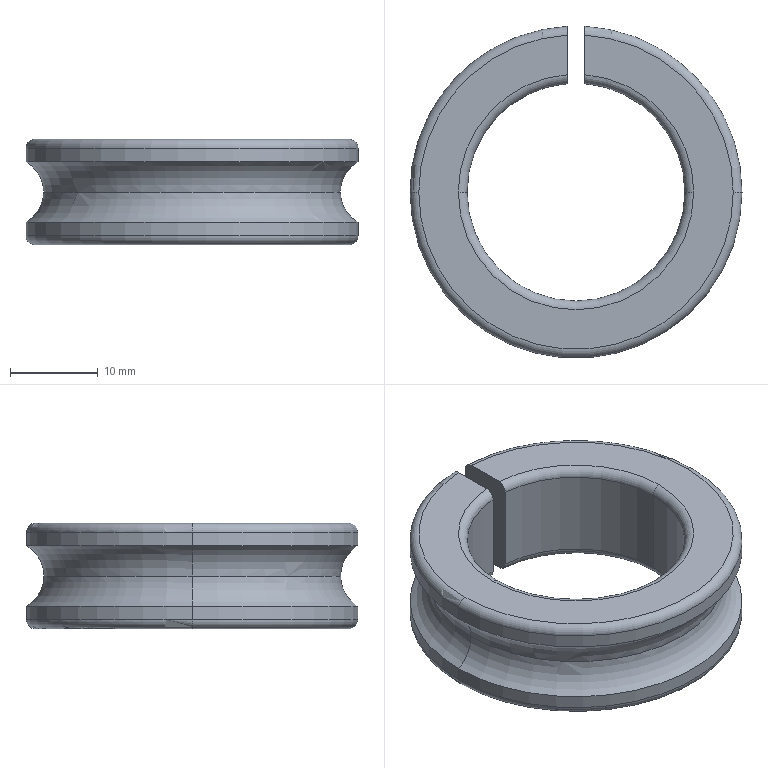Part | STEP file | 10000020543swp000-1 | 1 solid | 31 faces | box 37.8 x 37.774 x 12 mm | volume 6334 mm3 | torus 18 | cylinder 9 | plane 4 | commonest cylinder face diameters 37.8 x6 24.8 x3
STEP:
#1=CARTESIAN_POINT('',(-1.,16.87,0.));
#2=VERTEX_POINT('',#1);
#3=CARTESIAN_POINT('',(-1.,18.874,3.464));
#4=VERTEX_POINT('',#3);
#5=CARTESIAN_POINT('',(-1.,16.87,0.));
#6=CARTESIAN_POINT('',(-1.,16.87,0.3477));
#7=CARTESIAN_POINT('',(-1.,16.917,0.701));
#8=CARTESIAN_POINT('',(-1.,17.053,1.205));
#9=CARTESIAN_POINT('',(-1.,17.109,1.37));
#10=CARTESIAN_POINT('',(-1.,17.242,1.692));
#11=CARTESIAN_POINT('',(-1.,17.321,1.85));
#12=CARTESIAN_POINT('',(-1.,17.584,2.305));
#13=CARTESIAN_POINT('',(-1.,17.796,2.581));
#14=CARTESIAN_POINT('',(-1.,18.168,2.953));
#15=CARTESIAN_POINT('',(-1.,18.301,3.069));
#16=CARTESIAN_POINT('',(-1.,18.578,3.281));
#17=CARTESIAN_POINT('',(-1.,18.723,3.377));
#18=CARTESIAN_POINT('',(-1.,18.874,3.464));
#19=B_SPLINE_CURVE_WITH_KNOTS('',3,(#5,#6,#7,#8,#9,#10,#11,#12,#13,#14,#15,#16,#17,#18),.UNSPECIFIED.,.F.,.F.,(4,2,2,2,2,2,4),(0.002107,0.00315,0.003671,0.004193,0.005236,0.005757,0.006279),.UNSPECIFIED.);
#20=EDGE_CURVE('',#2,#4,#19,.T.);
#21=ORIENTED_EDGE('',*,*,#20,.F.);
#22=CARTESIAN_POINT('',(-16.9,0.,0.));
#23=VERTEX_POINT('',#22);
#24=CARTESIAN_POINT('',(0.,0.,0.));
#25=DIRECTION('',(0.,0.,1.));
#26=DIRECTION('',(1.,0.,0.));
#27=AXIS2_PLACEMENT_3D('',#24,#25,#26);
#28=CIRCLE('',#27,16.9);
#29=EDGE_CURVE('',#2,#23,#28,.T.);
#30=ORIENTED_EDGE('',*,*,#29,.T.);
#31=CARTESIAN_POINT('',(-18.9,0.,3.464));
#32=VERTEX_POINT('',#31);
#33=CARTESIAN_POINT('',(-20.9,0.,0.));
#34=DIRECTION('',(0.,1.,0.));
#35=DIRECTION('',(-1.,0.,0.));
#36=AXIS2_PLACEMENT_3D('',#33,#34,#35);
#37=CIRCLE('',#36,4.);
#38=EDGE_CURVE('',#32,#23,#37,.T.);
#39=ORIENTED_EDGE('',*,*,#38,.F.);
#40=CARTESIAN_POINT('',(0.,0.,3.464));
#41=DIRECTION('',(0.,0.,-1.));
#42=DIRECTION('',(-1.,0.,0.));
#43=AXIS2_PLACEMENT_3D('',#40,#41,#42);
#44=CIRCLE('',#43,18.9);
#45=EDGE_CURVE('',#32,#4,#44,.T.);
#46=ORIENTED_EDGE('',*,*,#45,.T.);
#47=EDGE_LOOP('',(#21,#30,#39,#46));
#48=FACE_OUTER_BOUND('',#47,.T.);
#49=CARTESIAN_POINT('',(0.,0.,0.));
#50=DIRECTION('',(0.,0.,1.));
#51=DIRECTION('',(1.,0.,0.));
#52=AXIS2_PLACEMENT_3D('',#49,#50,#51);
#53=TOROIDAL_SURFACE('',#52,20.9,4.);
#54=ADVANCED_FACE('',(#48),#53,.F.);
#55=CARTESIAN_POINT('',(18.9,0.,3.464));
#56=VERTEX_POINT('',#55);
#57=CARTESIAN_POINT('',(16.9,0.,0.));
#58=VERTEX_POINT('',#57);
#59=CARTESIAN_POINT('',(20.9,0.,0.));
#60=DIRECTION('',(0.,-1.,0.));
#61=DIRECTION('',(0.,0.,-1.));
#62=AXIS2_PLACEMENT_3D('',#59,#60,#61);
#63=CIRCLE('',#62,4.);
#64=EDGE_CURVE('',#56,#58,#63,.T.);
#65=ORIENTED_EDGE('',*,*,#64,.T.);
#66=CARTESIAN_POINT('',(1.,16.87,0.));
#67=VERTEX_POINT('',#66);
#68=CARTESIAN_POINT('',(0.,0.,0.));
#69=DIRECTION('',(0.,0.,1.));
#70=DIRECTION('',(1.,0.,0.));
#71=AXIS2_PLACEMENT_3D('',#68,#69,#70);
#72=CIRCLE('',#71,16.9);
#73=EDGE_CURVE('',#58,#67,#72,.T.);
#74=ORIENTED_EDGE('',*,*,#73,.T.);
#75=CARTESIAN_POINT('',(1.,18.874,3.464));
#76=VERTEX_POINT('',#75);
#77=CARTESIAN_POINT('',(1.,18.874,3.464));
#78=CARTESIAN_POINT('',(1.,18.569,3.289));
#79=CARTESIAN_POINT('',(1.,18.292,3.076));
#80=CARTESIAN_POINT('',(1.,17.922,2.706));
#81=CARTESIAN_POINT('',(1.,17.805,2.574));
#82=CARTESIAN_POINT('',(1.,17.591,2.296));
#83=CARTESIAN_POINT('',(1.,17.398,2.006));
#84=CARTESIAN_POINT('',(1.,17.243,1.694));
#85=CARTESIAN_POINT('',(1.,17.109,1.371));
#86=CARTESIAN_POINT('',(1.,17.052,1.203));
#87=CARTESIAN_POINT('',(1.,16.917,0.6983));
#88=CARTESIAN_POINT('',(1.,16.87,0.3515));
#89=CARTESIAN_POINT('',(1.,16.87,0.));
#90=B_SPLINE_CURVE_WITH_KNOTS('',3,(#77,#78,#79,#80,#81,#82,#83,#84,#85,#86,#87,#88,#89),.UNSPECIFIED.,.F.,.F.,(4,2,2,1,2,2,4),(0.01875,0.01979,0.02031,0.02084,0.02136,0.02188,0.02292),.UNSPECIFIED.);
#91=EDGE_CURVE('',#76,#67,#90,.T.);
#92=ORIENTED_EDGE('',*,*,#91,.F.);
#93=CARTESIAN_POINT('',(0.,0.,3.464));
#94=DIRECTION('',(0.,0.,-1.));
#95=DIRECTION('',(-1.,0.,0.));
#96=AXIS2_PLACEMENT_3D('',#93,#94,#95);
#97=CIRCLE('',#96,18.9);
#98=EDGE_CURVE('',#76,#56,#97,.T.);
#99=ORIENTED_EDGE('',*,*,#98,.T.);
#100=EDGE_LOOP('',(#65,#74,#92,#99));
#101=FACE_OUTER_BOUND('',#100,.T.);
#102=CARTESIAN_POINT('',(0.,0.,0.));
#103=DIRECTION('',(0.,0.,1.));
#104=DIRECTION('',(1.,0.,0.));
#105=AXIS2_PLACEMENT_3D('',#102,#103,#104);
#106=TOROIDAL_SURFACE('',#105,20.9,4.);
#107=ADVANCED_FACE('',(#101),#106,.F.);
#108=ORIENTED_EDGE('',*,*,#38,.T.);
#109=CARTESIAN_POINT('',(0.,0.,0.));
#110=DIRECTION('',(0.,0.,1.));
#111=DIRECTION('',(1.,0.,0.));
#112=AXIS2_PLACEMENT_3D('',#109,#110,#111);
#113=CIRCLE('',#112,16.9);
#114=EDGE_CURVE('',#23,#58,#113,.T.);
#115=ORIENTED_EDGE('',*,*,#114,.T.);
#116=ORIENTED_EDGE('',*,*,#64,.F.);
#117=CARTESIAN_POINT('',(0.,0.,3.464));
#118=DIRECTION('',(0.,0.,-1.));
#119=DIRECTION('',(-1.,0.,0.));
#120=AXIS2_PLACEMENT_3D('',#117,#118,#119);
#121=CIRCLE('',#120,18.9);
#122=EDGE_CURVE('',#56,#32,#121,.T.);
#123=ORIENTED_EDGE('',*,*,#122,.T.);
#124=EDGE_LOOP('',(#108,#115,#116,#123));
#125=FACE_OUTER_BOUND('',#124,.T.);
#126=CARTESIAN_POINT('',(0.,0.,0.));
#127=DIRECTION('',(0.,0.,1.));
#128=DIRECTION('',(1.,0.,0.));
#129=AXIS2_PLACEMENT_3D('',#126,#127,#128);
#130=TOROIDAL_SURFACE('',#129,20.9,4.);
#131=ADVANCED_FACE('',(#125),#130,.F.);
#132=CARTESIAN_POINT('',(-17.9,0.,-6.));
#133=VERTEX_POINT('',#132);
#134=CARTESIAN_POINT('',(-1.,17.872,-6.));
#135=VERTEX_POINT('',#134);
#136=CARTESIAN_POINT('',(0.,0.,-6.));
#137=DIRECTION('',(0.,0.,-1.));
#138=DIRECTION('',(1.,0.,0.));
#139=AXIS2_PLACEMENT_3D('',#136,#137,#138);
#140=CIRCLE('',#139,17.9);
#141=EDGE_CURVE('',#133,#135,#140,.T.);
#142=ORIENTED_EDGE('',*,*,#141,.F.);
#143=CARTESIAN_POINT('',(-18.9,0.,-5.));
#144=VERTEX_POINT('',#143);
#145=CARTESIAN_POINT('',(-17.9,0.,-5.));
#146=DIRECTION('',(0.,1.,0.));
#147=DIRECTION('',(-1.,0.,0.));
#148=AXIS2_PLACEMENT_3D('',#145,#146,#147);
#149=CIRCLE('',#148,1.);
#150=EDGE_CURVE('',#133,#144,#149,.T.);
#151=ORIENTED_EDGE('',*,*,#150,.T.);
#152=CARTESIAN_POINT('',(-1.,18.874,-5.));
#153=VERTEX_POINT('',#152);
#154=CARTESIAN_POINT('',(0.,0.,-5.));
#155=DIRECTION('',(0.,0.,1.));
#156=DIRECTION('',(1.,0.,0.));
#157=AXIS2_PLACEMENT_3D('',#154,#155,#156);
#158=CIRCLE('',#157,18.9);
#159=EDGE_CURVE('',#153,#144,#158,.T.);
#160=ORIENTED_EDGE('',*,*,#159,.F.);
#161=CARTESIAN_POINT('',(-1.,17.872,-6.));
#162=CARTESIAN_POINT('',(-1.,18.004,-6.));
#163=CARTESIAN_POINT('',(-1.,18.134,-5.974));
#164=CARTESIAN_POINT('',(-1.,18.376,-5.874));
#165=CARTESIAN_POINT('',(-1.,18.487,-5.8));
#166=CARTESIAN_POINT('',(-1.,18.765,-5.523));
#167=CARTESIAN_POINT('',(-1.,18.874,-5.264));
#168=CARTESIAN_POINT('',(-1.,18.874,-5.));
#169=B_SPLINE_CURVE_WITH_KNOTS('',3,(#161,#162,#163,#164,#165,#166,#167,#168),.UNSPECIFIED.,.F.,.F.,(4,2,2,4),(0.,0.0003908,0.0007817,0.001563),.UNSPECIFIED.);
#170=EDGE_CURVE('',#135,#153,#169,.T.);
#171=ORIENTED_EDGE('',*,*,#170,.F.);
#172=EDGE_LOOP('',(#142,#151,#160,#171));
#173=FACE_OUTER_BOUND('',#172,.T.);
#174=CARTESIAN_POINT('',(0.,0.,-5.));
#175=DIRECTION('',(0.,0.,1.));
#176=DIRECTION('',(1.,0.,0.));
#177=AXIS2_PLACEMENT_3D('',#174,#175,#176);
#178=TOROIDAL_SURFACE('',#177,17.9,1.);
#179=ADVANCED_FACE('',(#173),#178,.T.);
#180=ORIENTED_EDGE('',*,*,#150,.F.);
#181=CARTESIAN_POINT('',(17.9,0.,-6.));
#182=VERTEX_POINT('',#181);
#183=CARTESIAN_POINT('',(0.,0.,-6.));
#184=DIRECTION('',(0.,0.,-1.));
#185=DIRECTION('',(1.,0.,0.));
#186=AXIS2_PLACEMENT_3D('',#183,#184,#185);
#187=CIRCLE('',#186,17.9);
#188=EDGE_CURVE('',#182,#133,#187,.T.);
#189=ORIENTED_EDGE('',*,*,#188,.F.);
#190=CARTESIAN_POINT('',(18.9,0.,-5.));
#191=VERTEX_POINT('',#190);
#192=CARTESIAN_POINT('',(17.9,0.,-5.));
#193=DIRECTION('',(0.,-1.,0.));
#194=DIRECTION('',(0.,0.,-1.));
#195=AXIS2_PLACEMENT_3D('',#192,#193,#194);
#196=CIRCLE('',#195,1.);
#197=EDGE_CURVE('',#182,#191,#196,.T.);
#198=ORIENTED_EDGE('',*,*,#197,.T.);
#199=CARTESIAN_POINT('',(0.,0.,-5.));
#200=DIRECTION('',(0.,0.,1.));
#201=DIRECTION('',(1.,0.,0.));
#202=AXIS2_PLACEMENT_3D('',#199,#200,#201);
#203=CIRCLE('',#202,18.9);
#204=EDGE_CURVE('',#144,#191,#203,.T.);
#205=ORIENTED_EDGE('',*,*,#204,.F.);
#206=EDGE_LOOP('',(#180,#189,#198,#205));
#207=FACE_OUTER_BOUND('',#206,.T.);
#208=CARTESIAN_POINT('',(0.,0.,-5.));
#209=DIRECTION('',(0.,0.,1.));
#210=DIRECTION('',(1.,0.,0.));
#211=AXIS2_PLACEMENT_3D('',#208,#209,#210);
#212=TOROIDAL_SURFACE('',#211,17.9,1.);
#213=ADVANCED_FACE('',(#207),#212,.T.);
#214=CARTESIAN_POINT('',(-12.4,0.,-5.));
#215=VERTEX_POINT('',#214);
#216=CARTESIAN_POINT('',(-1.,12.36,-5.));
#217=VERTEX_POINT('',#216);
#218=CARTESIAN_POINT('',(0.,0.,-5.));
#219=DIRECTION('',(0.,0.,-1.));
#220=DIRECTION('',(1.,0.,0.));
#221=AXIS2_PLACEMENT_3D('',#218,#219,#220);
#222=CIRCLE('',#221,12.4);
#223=EDGE_CURVE('',#215,#217,#222,.T.);
#224=ORIENTED_EDGE('',*,*,#223,.F.);
#225=CARTESIAN_POINT('',(-13.4,0.,-6.));
#226=VERTEX_POINT('',#225);
#227=CARTESIAN_POINT('',(-13.4,0.,-5.));
#228=DIRECTION('',(0.,1.,0.));
#229=DIRECTION('',(-1.,0.,0.));
#230=AXIS2_PLACEMENT_3D('',#227,#228,#229);
#231=CIRCLE('',#230,1.);
#232=EDGE_CURVE('',#215,#226,#231,.T.);
#233=ORIENTED_EDGE('',*,*,#232,.T.);
#234=CARTESIAN_POINT('',(-1.,13.363,-6.));
#235=VERTEX_POINT('',#234);
#236=CARTESIAN_POINT('',(0.,0.,-6.));
#237=DIRECTION('',(0.,0.,1.));
#238=DIRECTION('',(1.,0.,0.));
#239=AXIS2_PLACEMENT_3D('',#236,#237,#238);
#240=CIRCLE('',#239,13.4);
#241=EDGE_CURVE('',#235,#226,#240,.T.);
#242=ORIENTED_EDGE('',*,*,#241,.F.);
#243=CARTESIAN_POINT('',(-1.,12.36,-5.));
#244=CARTESIAN_POINT('',(-1.,12.36,-5.132));
#245=CARTESIAN_POINT('',(-1.,12.386,-5.262));
#246=CARTESIAN_POINT('',(-1.,12.487,-5.504));
#247=CARTESIAN_POINT('',(-1.,12.561,-5.615));
#248=CARTESIAN_POINT('',(-1.,12.839,-5.892));
#249=CARTESIAN_POINT('',(-1.,13.098,-6.));
#250=CARTESIAN_POINT('',(-1.,13.363,-6.));
#251=B_SPLINE_CURVE_WITH_KNOTS('',3,(#243,#244,#245,#246,#247,#248,#249,#250),.UNSPECIFIED.,.F.,.F.,(4,2,2,4),(0.,0.0003911,0.0007822,0.001564),.UNSPECIFIED.);
#252=EDGE_CURVE('',#217,#235,#251,.T.);
#253=ORIENTED_EDGE('',*,*,#252,.F.);
#254=EDGE_LOOP('',(#224,#233,#242,#253));
#255=FACE_OUTER_BOUND('',#254,.T.);
#256=CARTESIAN_POINT('',(0.,0.,-5.));
#257=DIRECTION('',(0.,0.,1.));
#258=DIRECTION('',(1.,0.,0.));
#259=AXIS2_PLACEMENT_3D('',#256,#257,#258);
#260=TOROIDAL_SURFACE('',#259,13.4,1.);
#261=ADVANCED_FACE('',(#255),#260,.T.);
#262=ORIENTED_EDGE('',*,*,#232,.F.);
#263=CARTESIAN_POINT('',(12.4,0.,-5.));
#264=VERTEX_POINT('',#263);
#265=CARTESIAN_POINT('',(0.,0.,-5.));
#266=DIRECTION('',(0.,0.,-1.));
#267=DIRECTION('',(1.,0.,0.));
#268=AXIS2_PLACEMENT_3D('',#265,#266,#267);
#269=CIRCLE('',#268,12.4);
#270=EDGE_CURVE('',#264,#215,#269,.T.);
#271=ORIENTED_EDGE('',*,*,#270,.F.);
#272=CARTESIAN_POINT('',(13.4,0.,-6.));
#273=VERTEX_POINT('',#272);
#274=CARTESIAN_POINT('',(13.4,0.,-5.));
#275=DIRECTION('',(0.,-1.,0.));
#276=DIRECTION('',(0.,0.,-1.));
#277=AXIS2_PLACEMENT_3D('',#274,#275,#276);
#278=CIRCLE('',#277,1.);
#279=EDGE_CURVE('',#264,#273,#278,.T.);
#280=ORIENTED_EDGE('',*,*,#279,.T.);
#281=CARTESIAN_POINT('',(0.,0.,-6.));
#282=DIRECTION('',(0.,0.,1.));
#283=DIRECTION('',(1.,0.,0.));
#284=AXIS2_PLACEMENT_3D('',#281,#282,#283);
#285=CIRCLE('',#284,13.4);
#286=EDGE_CURVE('',#226,#273,#285,.T.);
#287=ORIENTED_EDGE('',*,*,#286,.F.);
#288=EDGE_LOOP('',(#262,#271,#280,#287));
#289=FACE_OUTER_BOUND('',#288,.T.);
#290=CARTESIAN_POINT('',(0.,0.,-5.));
#291=DIRECTION('',(0.,0.,1.));
#292=DIRECTION('',(1.,0.,0.));
#293=AXIS2_PLACEMENT_3D('',#290,#291,#292);
#294=TOROIDAL_SURFACE('',#293,13.4,1.);
#295=ADVANCED_FACE('',(#289),#294,.T.);
#296=CARTESIAN_POINT('',(-13.4,0.,6.));
#297=VERTEX_POINT('',#296);
#298=CARTESIAN_POINT('',(-1.,13.363,6.));
#299=VERTEX_POINT('',#298);
#300=CARTESIAN_POINT('',(0.,0.,6.));
#301=DIRECTION('',(0.,0.,-1.));
#302=DIRECTION('',(1.,0.,0.));
#303=AXIS2_PLACEMENT_3D('',#300,#301,#302);
#304=CIRCLE('',#303,13.4);
#305=EDGE_CURVE('',#297,#299,#304,.T.);
#306=ORIENTED_EDGE('',*,*,#305,.F.);
#307=CARTESIAN_POINT('',(-12.4,0.,5.));
#308=VERTEX_POINT('',#307);
#309=CARTESIAN_POINT('',(-13.4,0.,5.));
#310=DIRECTION('',(0.,1.,0.));
#311=DIRECTION('',(-1.,0.,0.));
#312=AXIS2_PLACEMENT_3D('',#309,#310,#311);
#313=CIRCLE('',#312,1.);
#314=EDGE_CURVE('',#297,#308,#313,.T.);
#315=ORIENTED_EDGE('',*,*,#314,.T.);
#316=CARTESIAN_POINT('',(-1.,12.36,5.));
#317=VERTEX_POINT('',#316);
#318=CARTESIAN_POINT('',(0.,0.,5.));
#319=DIRECTION('',(0.,0.,1.));
#320=DIRECTION('',(1.,0.,0.));
#321=AXIS2_PLACEMENT_3D('',#318,#319,#320);
#322=CIRCLE('',#321,12.4);
#323=EDGE_CURVE('',#317,#308,#322,.T.);
#324=ORIENTED_EDGE('',*,*,#323,.F.);
#325=CARTESIAN_POINT('',(-1.,13.363,6.));
#326=CARTESIAN_POINT('',(-1.,13.23,6.));
#327=CARTESIAN_POINT('',(-1.,13.101,5.974));
#328=CARTESIAN_POINT('',(-1.,12.858,5.874));
#329=CARTESIAN_POINT('',(-1.,12.747,5.8));
#330=CARTESIAN_POINT('',(-1.,12.469,5.524));
#331=CARTESIAN_POINT('',(-1.,12.36,5.265));
#332=CARTESIAN_POINT('',(-1.,12.36,5.));
#333=B_SPLINE_CURVE_WITH_KNOTS('',3,(#325,#326,#327,#328,#329,#330,#331,#332),.UNSPECIFIED.,.F.,.F.,(4,2,2,4),(0.,0.0003911,0.0007822,0.001564),.UNSPECIFIED.);
#334=EDGE_CURVE('',#299,#317,#333,.T.);
#335=ORIENTED_EDGE('',*,*,#334,.F.);
#336=EDGE_LOOP('',(#306,#315,#324,#335));
#337=FACE_OUTER_BOUND('',#336,.T.);
#338=CARTESIAN_POINT('',(0.,0.,5.));
#339=DIRECTION('',(0.,0.,1.));
#340=DIRECTION('',(1.,0.,0.));
#341=AXIS2_PLACEMENT_3D('',#338,#339,#340);
#342=TOROIDAL_SURFACE('',#341,13.4,1.);
#343=ADVANCED_FACE('',(#337),#342,.T.);
#344=ORIENTED_EDGE('',*,*,#314,.F.);
#345=CARTESIAN_POINT('',(13.4,0.,6.));
#346=VERTEX_POINT('',#345);
#347=CARTESIAN_POINT('',(0.,0.,6.));
#348=DIRECTION('',(0.,0.,-1.));
#349=DIRECTION('',(1.,0.,0.));
#350=AXIS2_PLACEMENT_3D('',#347,#348,#349);
#351=CIRCLE('',#350,13.4);
#352=EDGE_CURVE('',#346,#297,#351,.T.);
#353=ORIENTED_EDGE('',*,*,#352,.F.);
#354=CARTESIAN_POINT('',(12.4,0.,5.));
#355=VERTEX_POINT('',#354);
#356=CARTESIAN_POINT('',(13.4,0.,5.));
#357=DIRECTION('',(0.,-1.,0.));
#358=DIRECTION('',(0.,0.,-1.));
#359=AXIS2_PLACEMENT_3D('',#356,#357,#358);
#360=CIRCLE('',#359,1.);
#361=EDGE_CURVE('',#346,#355,#360,.T.);
#362=ORIENTED_EDGE('',*,*,#361,.T.);
#363=CARTESIAN_POINT('',(0.,0.,5.));
#364=DIRECTION('',(0.,0.,1.));
#365=DIRECTION('',(1.,0.,0.));
#366=AXIS2_PLACEMENT_3D('',#363,#364,#365);
#367=CIRCLE('',#366,12.4);
#368=EDGE_CURVE('',#308,#355,#367,.T.);
#369=ORIENTED_EDGE('',*,*,#368,.F.);
#370=EDGE_LOOP('',(#344,#353,#362,#369));
#371=FACE_OUTER_BOUND('',#370,.T.);
#372=CARTESIAN_POINT('',(0.,0.,5.));
#373=DIRECTION('',(0.,0.,1.));
#374=DIRECTION('',(1.,0.,0.));
#375=AXIS2_PLACEMENT_3D('',#372,#373,#374);
#376=TOROIDAL_SURFACE('',#375,13.4,1.);
#377=ADVANCED_FACE('',(#371),#376,.T.);
#378=CARTESIAN_POINT('',(-18.9,0.,5.));
#379=VERTEX_POINT('',#378);
#380=CARTESIAN_POINT('',(-1.,18.874,5.));
#381=VERTEX_POINT('',#380);
#382=CARTESIAN_POINT('',(0.,0.,5.));
#383=DIRECTION('',(0.,0.,-1.));
#384=DIRECTION('',(1.,0.,0.));
#385=AXIS2_PLACEMENT_3D('',#382,#383,#384);
#386=CIRCLE('',#385,18.9);
#387=EDGE_CURVE('',#379,#381,#386,.T.);
#388=ORIENTED_EDGE('',*,*,#387,.F.);
#389=CARTESIAN_POINT('',(-17.9,0.,6.));
#390=VERTEX_POINT('',#389);
#391=CARTESIAN_POINT('',(-17.9,0.,5.));
#392=DIRECTION('',(0.,1.,0.));
#393=DIRECTION('',(-1.,0.,0.));
#394=AXIS2_PLACEMENT_3D('',#391,#392,#393);
#395=CIRCLE('',#394,1.);
#396=EDGE_CURVE('',#379,#390,#395,.T.);
#397=ORIENTED_EDGE('',*,*,#396,.T.);
#398=CARTESIAN_POINT('',(-1.,17.872,6.));
#399=VERTEX_POINT('',#398);
#400=CARTESIAN_POINT('',(0.,0.,6.));
#401=DIRECTION('',(0.,0.,1.));
#402=DIRECTION('',(1.,0.,0.));
#403=AXIS2_PLACEMENT_3D('',#400,#401,#402);
#404=CIRCLE('',#403,17.9);
#405=EDGE_CURVE('',#399,#390,#404,.T.);
#406=ORIENTED_EDGE('',*,*,#405,.F.);
#407=CARTESIAN_POINT('',(-1.,18.874,5.));
#408=CARTESIAN_POINT('',(-1.,18.874,5.132));
#409=CARTESIAN_POINT('',(-1.,18.847,5.262));
#410=CARTESIAN_POINT('',(-1.,18.747,5.504));
#411=CARTESIAN_POINT('',(-1.,18.673,5.615));
#412=CARTESIAN_POINT('',(-1.,18.396,5.892));
#413=CARTESIAN_POINT('',(-1.,18.136,6.));
#414=CARTESIAN_POINT('',(-1.,17.872,6.));
#415=B_SPLINE_CURVE_WITH_KNOTS('',3,(#407,#408,#409,#410,#411,#412,#413,#414),.UNSPECIFIED.,.F.,.F.,(4,2,2,4),(0.,0.0003908,0.0007817,0.001563),.UNSPECIFIED.);
#416=EDGE_CURVE('',#381,#399,#415,.T.);
#417=ORIENTED_EDGE('',*,*,#416,.F.);
#418=EDGE_LOOP('',(#388,#397,#406,#417));
#419=FACE_OUTER_BOUND('',#418,.T.);
#420=CARTESIAN_POINT('',(0.,0.,5.));
#421=DIRECTION('',(0.,0.,1.));
#422=DIRECTION('',(1.,0.,0.));
#423=AXIS2_PLACEMENT_3D('',#420,#421,#422);
#424=TOROIDAL_SURFACE('',#423,17.9,1.);
#425=ADVANCED_FACE('',(#419),#424,.T.);
#426=ORIENTED_EDGE('',*,*,#396,.F.);
#427=CARTESIAN_POINT('',(18.9,0.,5.));
#428=VERTEX_POINT('',#427);
#429=CARTESIAN_POINT('',(0.,0.,5.));
#430=DIRECTION('',(0.,0.,-1.));
#431=DIRECTION('',(1.,0.,0.));
#432=AXIS2_PLACEMENT_3D('',#429,#430,#431);
#433=CIRCLE('',#432,18.9);
#434=EDGE_CURVE('',#428,#379,#433,.T.);
#435=ORIENTED_EDGE('',*,*,#434,.F.);
#436=CARTESIAN_POINT('',(17.9,0.,6.));
#437=VERTEX_POINT('',#436);
#438=CARTESIAN_POINT('',(17.9,0.,5.));
#439=DIRECTION('',(0.,-1.,0.));
#440=DIRECTION('',(0.,0.,-1.));
#441=AXIS2_PLACEMENT_3D('',#438,#439,#440);
#442=CIRCLE('',#441,1.);
#443=EDGE_CURVE('',#428,#437,#442,.T.);
#444=ORIENTED_EDGE('',*,*,#443,.T.);
#445=CARTESIAN_POINT('',(0.,0.,6.));
#446=DIRECTION('',(0.,0.,1.));
#447=DIRECTION('',(1.,0.,0.));
#448=AXIS2_PLACEMENT_3D('',#445,#446,#447);
#449=CIRCLE('',#448,17.9);
#450=EDGE_CURVE('',#390,#437,#449,.T.);
#451=ORIENTED_EDGE('',*,*,#450,.F.);
#452=EDGE_LOOP('',(#426,#435,#444,#451));
#453=FACE_OUTER_BOUND('',#452,.T.);
#454=CARTESIAN_POINT('',(0.,0.,5.));
#455=DIRECTION('',(0.,0.,1.));
#456=DIRECTION('',(1.,0.,0.));
#457=AXIS2_PLACEMENT_3D('',#454,#455,#456);
#458=TOROIDAL_SURFACE('',#457,17.9,1.);
#459=ADVANCED_FACE('',(#453),#458,.T.);
#460=ORIENTED_EDGE('',*,*,#114,.F.);
#461=CARTESIAN_POINT('',(-18.9,0.,-3.464));
#462=VERTEX_POINT('',#461);
#463=CARTESIAN_POINT('',(-20.9,0.,0.));
#464=DIRECTION('',(0.,1.,0.));
#465=DIRECTION('',(-1.,0.,0.));
#466=AXIS2_PLACEMENT_3D('',#463,#464,#465);
#467=CIRCLE('',#466,4.);
#468=EDGE_CURVE('',#23,#462,#467,.T.);
#469=ORIENTED_EDGE('',*,*,#468,.T.);
#470=CARTESIAN_POINT('',(18.9,0.,-3.464));
#471=VERTEX_POINT('',#470);
#472=CARTESIAN_POINT('',(0.,0.,-3.464));
#473=DIRECTION('',(0.,0.,1.));
#474=DIRECTION('',(1.,0.,0.));
#475=AXIS2_PLACEMENT_3D('',#472,#473,#474);
#476=CIRCLE('',#475,18.9);
#477=EDGE_CURVE('',#462,#471,#476,.T.);
#478=ORIENTED_EDGE('',*,*,#477,.T.);
#479=CARTESIAN_POINT('',(20.9,0.,0.));
#480=DIRECTION('',(0.,-1.,0.));
#481=DIRECTION('',(0.,0.,-1.));
#482=AXIS2_PLACEMENT_3D('',#479,#480,#481);
#483=CIRCLE('',#482,4.);
#484=EDGE_CURVE('',#58,#471,#483,.T.);
#485=ORIENTED_EDGE('',*,*,#484,.F.);
#486=EDGE_LOOP('',(#460,#469,#478,#485));
#487=FACE_OUTER_BOUND('',#486,.T.);
#488=CARTESIAN_POINT('',(0.,0.,0.));
#489=DIRECTION('',(0.,0.,1.));
#490=DIRECTION('',(1.,0.,0.));
#491=AXIS2_PLACEMENT_3D('',#488,#489,#490);
#492=TOROIDAL_SURFACE('',#491,20.9,4.);
#493=ADVANCED_FACE('',(#487),#492,.F.);
#494=ORIENTED_EDGE('',*,*,#73,.F.);
#495=ORIENTED_EDGE('',*,*,#484,.T.);
#496=CARTESIAN_POINT('',(1.,18.874,-3.464));
#497=VERTEX_POINT('',#496);
#498=CARTESIAN_POINT('',(0.,0.,-3.464));
#499=DIRECTION('',(0.,0.,1.));
#500=DIRECTION('',(1.,0.,0.));
#501=AXIS2_PLACEMENT_3D('',#498,#499,#500);
#502=CIRCLE('',#501,18.9);
#503=EDGE_CURVE('',#471,#497,#502,.T.);
#504=ORIENTED_EDGE('',*,*,#503,.T.);
#505=CARTESIAN_POINT('',(1.,16.87,0.));
#506=CARTESIAN_POINT('',(1.,16.87,-0.3513));
#507=CARTESIAN_POINT('',(1.,16.916,-0.6956));
#508=CARTESIAN_POINT('',(1.,17.051,-1.202));
#509=CARTESIAN_POINT('',(1.,17.108,-1.369));
#510=CARTESIAN_POINT('',(1.,17.243,-1.693));
#511=CARTESIAN_POINT('',(1.,17.32,-1.85));
#512=CARTESIAN_POINT('',(1.,17.585,-2.307));
#513=CARTESIAN_POINT('',(1.,17.798,-2.583));
#514=CARTESIAN_POINT('',(1.,18.168,-2.952));
#515=CARTESIAN_POINT('',(1.,18.301,-3.068));
#516=CARTESIAN_POINT('',(1.,18.578,-3.281));
#517=CARTESIAN_POINT('',(1.,18.723,-3.377));
#518=CARTESIAN_POINT('',(1.,18.874,-3.464));
#519=B_SPLINE_CURVE_WITH_KNOTS('',3,(#505,#506,#507,#508,#509,#510,#511,#512,#513,#514,#515,#516,#517,#518),.UNSPECIFIED.,.F.,.F.,(4,2,2,2,2,2,4),(0.02292,0.02396,0.02448,0.025,0.02605,0.02657,0.02709),.UNSPECIFIED.);
#520=EDGE_CURVE('',#67,#497,#519,.T.);
#521=ORIENTED_EDGE('',*,*,#520,.F.);
#522=EDGE_LOOP('',(#494,#495,#504,#521));
#523=FACE_OUTER_BOUND('',#522,.T.);
#524=CARTESIAN_POINT('',(0.,0.,0.));
#525=DIRECTION('',(0.,0.,1.));
#526=DIRECTION('',(1.,0.,0.));
#527=AXIS2_PLACEMENT_3D('',#524,#525,#526);
#528=TOROIDAL_SURFACE('',#527,20.9,4.);
#529=ADVANCED_FACE('',(#523),#528,.F.);
#530=ORIENTED_EDGE('',*,*,#368,.T.);
#531=CARTESIAN_POINT('',(12.4,0.,6.));
#532=DIRECTION('',(0.,0.,-1.));
#533=VECTOR('',#532,1000.);
#534=LINE('',#531,#533);
#535=EDGE_CURVE('',#355,#264,#534,.T.);
#536=ORIENTED_EDGE('',*,*,#535,.T.);
#537=ORIENTED_EDGE('',*,*,#270,.T.);
#538=CARTESIAN_POINT('',(-12.4,0.,6.));
#539=DIRECTION('',(0.,0.,-1.));
#540=VECTOR('',#539,1000.);
#541=LINE('',#538,#540);
#542=EDGE_CURVE('',#308,#215,#541,.T.);
#543=ORIENTED_EDGE('',*,*,#542,.F.);
#544=EDGE_LOOP('',(#530,#536,#537,#543));
#545=FACE_OUTER_BOUND('',#544,.T.);
#546=CARTESIAN_POINT('',(0.,0.,6.));
#547=DIRECTION('',(0.,0.,-1.));
#548=DIRECTION('',(-1.,0.,0.));
#549=AXIS2_PLACEMENT_3D('',#546,#547,#548);
#550=CYLINDRICAL_SURFACE('',#549,12.4);
#551=ADVANCED_FACE('',(#545),#550,.F.);
#552=ORIENTED_EDGE('',*,*,#323,.T.);
#553=ORIENTED_EDGE('',*,*,#542,.T.);
#554=ORIENTED_EDGE('',*,*,#223,.T.);
#555=CARTESIAN_POINT('',(-1.,12.36,6.));
#556=DIRECTION('',(0.,0.,-1.));
#557=VECTOR('',#556,1000.);
#558=LINE('',#555,#557);
#559=EDGE_CURVE('',#317,#217,#558,.T.);
#560=ORIENTED_EDGE('',*,*,#559,.F.);
#561=EDGE_LOOP('',(#552,#553,#554,#560));
#562=FACE_OUTER_BOUND('',#561,.T.);
#563=CARTESIAN_POINT('',(0.,0.,6.));
#564=DIRECTION('',(0.,0.,-1.));
#565=DIRECTION('',(-1.,0.,0.));
#566=AXIS2_PLACEMENT_3D('',#563,#564,#565);
#567=CYLINDRICAL_SURFACE('',#566,12.4);
#568=ADVANCED_FACE('',(#562),#567,.F.);
#569=ORIENTED_EDGE('',*,*,#503,.F.);
#570=CARTESIAN_POINT('',(18.9,0.,6.));
#571=DIRECTION('',(0.,0.,-1.));
#572=VECTOR('',#571,1000.);
#573=LINE('',#570,#572);
#574=EDGE_CURVE('',#471,#191,#573,.T.);
#575=ORIENTED_EDGE('',*,*,#574,.T.);
#576=CARTESIAN_POINT('',(1.,18.874,-5.));
#577=VERTEX_POINT('',#576);
#578=CARTESIAN_POINT('',(0.,0.,-5.));
#579=DIRECTION('',(0.,0.,1.));
#580=DIRECTION('',(1.,0.,0.));
#581=AXIS2_PLACEMENT_3D('',#578,#579,#580);
#582=CIRCLE('',#581,18.9);
#583=EDGE_CURVE('',#191,#577,#582,.T.);
#584=ORIENTED_EDGE('',*,*,#583,.T.);
#585=CARTESIAN_POINT('',(1.,18.874,6.));
#586=DIRECTION('',(0.,0.,-1.));
#587=VECTOR('',#586,1000.);
#588=LINE('',#585,#587);
#589=EDGE_CURVE('',#497,#577,#588,.T.);
#590=ORIENTED_EDGE('',*,*,#589,.F.);
#591=EDGE_LOOP('',(#569,#575,#584,#590));
#592=FACE_OUTER_BOUND('',#591,.T.);
#593=CARTESIAN_POINT('',(0.,0.,6.));
#594=DIRECTION('',(0.,0.,-1.));
#595=DIRECTION('',(-1.,0.,0.));
#596=AXIS2_PLACEMENT_3D('',#593,#594,#595);
#597=CYLINDRICAL_SURFACE('',#596,18.9);
#598=ADVANCED_FACE('',(#592),#597,.T.);
#599=ORIENTED_EDGE('',*,*,#574,.F.);
#600=ORIENTED_EDGE('',*,*,#477,.F.);
#601=CARTESIAN_POINT('',(-18.9,0.,6.));
#602=DIRECTION('',(0.,0.,-1.));
#603=VECTOR('',#602,1000.);
#604=LINE('',#601,#603);
#605=EDGE_CURVE('',#462,#144,#604,.T.);
#606=ORIENTED_EDGE('',*,*,#605,.T.);
#607=ORIENTED_EDGE('',*,*,#204,.T.);
#608=EDGE_LOOP('',(#599,#600,#606,#607));
#609=FACE_OUTER_BOUND('',#608,.T.);
#610=CARTESIAN_POINT('',(0.,0.,6.));
#611=DIRECTION('',(0.,0.,-1.));
#612=DIRECTION('',(-1.,0.,0.));
#613=AXIS2_PLACEMENT_3D('',#610,#611,#612);
#614=CYLINDRICAL_SURFACE('',#613,18.9);
#615=ADVANCED_FACE('',(#609),#614,.T.);
#616=CARTESIAN_POINT('',(1.,18.874,5.));
#617=VERTEX_POINT('',#616);
#618=CARTESIAN_POINT('',(0.,0.,5.));
#619=DIRECTION('',(0.,0.,-1.));
#620=DIRECTION('',(1.,0.,0.));
#621=AXIS2_PLACEMENT_3D('',#618,#619,#620);
#622=CIRCLE('',#621,18.9);
#623=EDGE_CURVE('',#617,#428,#622,.T.);
#624=ORIENTED_EDGE('',*,*,#623,.T.);
#625=CARTESIAN_POINT('',(18.9,0.,6.));
#626=DIRECTION('',(0.,0.,-1.));
#627=VECTOR('',#626,1000.);
#628=LINE('',#625,#627);
#629=EDGE_CURVE('',#428,#56,#628,.T.);
#630=ORIENTED_EDGE('',*,*,#629,.T.);
#631=ORIENTED_EDGE('',*,*,#98,.F.);
#632=CARTESIAN_POINT('',(1.,18.874,6.));
#633=DIRECTION('',(0.,0.,-1.));
#634=VECTOR('',#633,1000.);
#635=LINE('',#632,#634);
#636=EDGE_CURVE('',#617,#76,#635,.T.);
#637=ORIENTED_EDGE('',*,*,#636,.F.);
#638=EDGE_LOOP('',(#624,#630,#631,#637));
#639=FACE_OUTER_BOUND('',#638,.T.);
#640=CARTESIAN_POINT('',(0.,0.,6.));
#641=DIRECTION('',(0.,0.,-1.));
#642=DIRECTION('',(-1.,0.,0.));
#643=AXIS2_PLACEMENT_3D('',#640,#641,#642);
#644=CYLINDRICAL_SURFACE('',#643,18.9);
#645=ADVANCED_FACE('',(#639),#644,.T.);
#646=ORIENTED_EDGE('',*,*,#629,.F.);
#647=ORIENTED_EDGE('',*,*,#434,.T.);
#648=CARTESIAN_POINT('',(-18.9,0.,6.));
#649=DIRECTION('',(0.,0.,-1.));
#650=VECTOR('',#649,1000.);
#651=LINE('',#648,#650);
#652=EDGE_CURVE('',#379,#32,#651,.T.);
#653=ORIENTED_EDGE('',*,*,#652,.T.);
#654=ORIENTED_EDGE('',*,*,#122,.F.);
#655=EDGE_LOOP('',(#646,#647,#653,#654));
#656=FACE_OUTER_BOUND('',#655,.T.);
#657=CARTESIAN_POINT('',(0.,0.,6.));
#658=DIRECTION('',(0.,0.,-1.));
#659=DIRECTION('',(-1.,0.,0.));
#660=AXIS2_PLACEMENT_3D('',#657,#658,#659);
#661=CYLINDRICAL_SURFACE('',#660,18.9);
#662=ADVANCED_FACE('',(#656),#661,.T.);
#663=ORIENTED_EDGE('',*,*,#652,.F.);
#664=ORIENTED_EDGE('',*,*,#387,.T.);
#665=CARTESIAN_POINT('',(-1.,18.874,6.));
#666=DIRECTION('',(0.,0.,-1.));
#667=VECTOR('',#666,1000.);
#668=LINE('',#665,#667);
#669=EDGE_CURVE('',#381,#4,#668,.T.);
#670=ORIENTED_EDGE('',*,*,#669,.T.);
#671=ORIENTED_EDGE('',*,*,#45,.F.);
#672=EDGE_LOOP('',(#663,#664,#670,#671));
#673=FACE_OUTER_BOUND('',#672,.T.);
#674=CARTESIAN_POINT('',(0.,0.,6.));
#675=DIRECTION('',(0.,0.,-1.));
#676=DIRECTION('',(-1.,0.,0.));
#677=AXIS2_PLACEMENT_3D('',#674,#675,#676);
#678=CYLINDRICAL_SURFACE('',#677,18.9);
#679=ADVANCED_FACE('',(#673),#678,.T.);
#680=ORIENTED_EDGE('',*,*,#605,.F.);
#681=CARTESIAN_POINT('',(-1.,18.874,-3.464));
#682=VERTEX_POINT('',#681);
#683=CARTESIAN_POINT('',(0.,0.,-3.464));
#684=DIRECTION('',(0.,0.,1.));
#685=DIRECTION('',(1.,0.,0.));
#686=AXIS2_PLACEMENT_3D('',#683,#684,#685);
#687=CIRCLE('',#686,18.9);
#688=EDGE_CURVE('',#682,#462,#687,.T.);
#689=ORIENTED_EDGE('',*,*,#688,.F.);
#690=CARTESIAN_POINT('',(-1.,18.874,6.));
#691=DIRECTION('',(0.,0.,-1.));
#692=VECTOR('',#691,1000.);
#693=LINE('',#690,#692);
#694=EDGE_CURVE('',#682,#153,#693,.T.);
#695=ORIENTED_EDGE('',*,*,#694,.T.);
#696=ORIENTED_EDGE('',*,*,#159,.T.);
#697=EDGE_LOOP('',(#680,#689,#695,#696));
#698=FACE_OUTER_BOUND('',#697,.T.);
#699=CARTESIAN_POINT('',(0.,0.,6.));
#700=DIRECTION('',(0.,0.,-1.));
#701=DIRECTION('',(-1.,0.,0.));
#702=AXIS2_PLACEMENT_3D('',#699,#700,#701);
#703=CYLINDRICAL_SURFACE('',#702,18.9);
#704=ADVANCED_FACE('',(#698),#703,.T.);
#705=CARTESIAN_POINT('',(-1.,18.874,6.));
#706=DIRECTION('',(0.,1.,0.));
#707=VECTOR('',#706,1000.);
#708=LINE('',#705,#707);
#709=EDGE_CURVE('',#299,#399,#708,.T.);
#710=ORIENTED_EDGE('',*,*,#709,.T.);
#711=ORIENTED_EDGE('',*,*,#405,.T.);
#712=ORIENTED_EDGE('',*,*,#450,.T.);
#713=CARTESIAN_POINT('',(1.,17.872,6.));
#714=VERTEX_POINT('',#713);
#715=CARTESIAN_POINT('',(0.,0.,6.));
#716=DIRECTION('',(0.,0.,1.));
#717=DIRECTION('',(1.,0.,0.));
#718=AXIS2_PLACEMENT_3D('',#715,#716,#717);
#719=CIRCLE('',#718,17.9);
#720=EDGE_CURVE('',#437,#714,#719,.T.);
#721=ORIENTED_EDGE('',*,*,#720,.T.);
#722=CARTESIAN_POINT('',(1.,13.363,6.));
#723=VERTEX_POINT('',#722);
#724=CARTESIAN_POINT('',(1.,18.874,6.));
#725=DIRECTION('',(0.,-1.,0.));
#726=VECTOR('',#725,1000.);
#727=LINE('',#724,#726);
#728=EDGE_CURVE('',#714,#723,#727,.T.);
#729=ORIENTED_EDGE('',*,*,#728,.T.);
#730=CARTESIAN_POINT('',(0.,0.,6.));
#731=DIRECTION('',(0.,0.,-1.));
#732=DIRECTION('',(1.,0.,0.));
#733=AXIS2_PLACEMENT_3D('',#730,#731,#732);
#734=CIRCLE('',#733,13.4);
#735=EDGE_CURVE('',#723,#346,#734,.T.);
#736=ORIENTED_EDGE('',*,*,#735,.T.);
#737=ORIENTED_EDGE('',*,*,#352,.T.);
#738=ORIENTED_EDGE('',*,*,#305,.T.);
#739=EDGE_LOOP('',(#710,#711,#712,#721,#729,#736,#737,#738));
#740=FACE_OUTER_BOUND('',#739,.T.);
#741=CARTESIAN_POINT('',(0.,0.,6.));
#742=DIRECTION('',(0.,0.,1.));
#743=DIRECTION('',(1.,0.,0.));
#744=AXIS2_PLACEMENT_3D('',#741,#742,#743);
#745=PLANE('',#744);
#746=ADVANCED_FACE('',(#740),#745,.T.);
#747=CARTESIAN_POINT('',(-1.,18.874,-6.));
#748=DIRECTION('',(0.,1.,0.));
#749=VECTOR('',#748,1000.);
#750=LINE('',#747,#749);
#751=EDGE_CURVE('',#235,#135,#750,.T.);
#752=ORIENTED_EDGE('',*,*,#751,.F.);
#753=ORIENTED_EDGE('',*,*,#241,.T.);
#754=ORIENTED_EDGE('',*,*,#286,.T.);
#755=CARTESIAN_POINT('',(1.,13.363,-6.));
#756=VERTEX_POINT('',#755);
#757=CARTESIAN_POINT('',(0.,0.,-6.));
#758=DIRECTION('',(0.,0.,1.));
#759=DIRECTION('',(1.,0.,0.));
#760=AXIS2_PLACEMENT_3D('',#757,#758,#759);
#761=CIRCLE('',#760,13.4);
#762=EDGE_CURVE('',#273,#756,#761,.T.);
#763=ORIENTED_EDGE('',*,*,#762,.T.);
#764=CARTESIAN_POINT('',(1.,17.872,-6.));
#765=VERTEX_POINT('',#764);
#766=CARTESIAN_POINT('',(1.,18.874,-6.));
#767=DIRECTION('',(0.,-1.,0.));
#768=VECTOR('',#767,1000.);
#769=LINE('',#766,#768);
#770=EDGE_CURVE('',#765,#756,#769,.T.);
#771=ORIENTED_EDGE('',*,*,#770,.F.);
#772=CARTESIAN_POINT('',(0.,0.,-6.));
#773=DIRECTION('',(0.,0.,-1.));
#774=DIRECTION('',(1.,0.,0.));
#775=AXIS2_PLACEMENT_3D('',#772,#773,#774);
#776=CIRCLE('',#775,17.9);
#777=EDGE_CURVE('',#765,#182,#776,.T.);
#778=ORIENTED_EDGE('',*,*,#777,.T.);
#779=ORIENTED_EDGE('',*,*,#188,.T.);
#780=ORIENTED_EDGE('',*,*,#141,.T.);
#781=EDGE_LOOP('',(#752,#753,#754,#763,#771,#778,#779,#780));
#782=FACE_OUTER_BOUND('',#781,.T.);
#783=CARTESIAN_POINT('',(0.,0.,-6.));
#784=DIRECTION('',(0.,0.,1.));
#785=DIRECTION('',(1.,0.,0.));
#786=AXIS2_PLACEMENT_3D('',#783,#784,#785);
#787=PLANE('',#786);
#788=ADVANCED_FACE('',(#782),#787,.F.);
#789=ORIENTED_EDGE('',*,*,#535,.F.);
#790=CARTESIAN_POINT('',(1.,12.36,5.));
#791=VERTEX_POINT('',#790);
#792=CARTESIAN_POINT('',(0.,0.,5.));
#793=DIRECTION('',(0.,0.,1.));
#794=DIRECTION('',(1.,0.,0.));
#795=AXIS2_PLACEMENT_3D('',#792,#793,#794);
#796=CIRCLE('',#795,12.4);
#797=EDGE_CURVE('',#355,#791,#796,.T.);
#798=ORIENTED_EDGE('',*,*,#797,.T.);
#799=CARTESIAN_POINT('',(1.,12.36,-5.));
#800=VERTEX_POINT('',#799);
#801=CARTESIAN_POINT('',(1.,12.36,6.));
#802=DIRECTION('',(0.,0.,-1.));
#803=VECTOR('',#802,1000.);
#804=LINE('',#801,#803);
#805=EDGE_CURVE('',#791,#800,#804,.T.);
#806=ORIENTED_EDGE('',*,*,#805,.T.);
#807=CARTESIAN_POINT('',(0.,0.,-5.));
#808=DIRECTION('',(0.,0.,-1.));
#809=DIRECTION('',(1.,0.,0.));
#810=AXIS2_PLACEMENT_3D('',#807,#808,#809);
#811=CIRCLE('',#810,12.4);
#812=EDGE_CURVE('',#800,#264,#811,.T.);
#813=ORIENTED_EDGE('',*,*,#812,.T.);
#814=EDGE_LOOP('',(#789,#798,#806,#813));
#815=FACE_OUTER_BOUND('',#814,.T.);
#816=CARTESIAN_POINT('',(0.,0.,6.));
#817=DIRECTION('',(0.,0.,-1.));
#818=DIRECTION('',(-1.,0.,0.));
#819=AXIS2_PLACEMENT_3D('',#816,#817,#818);
#820=CYLINDRICAL_SURFACE('',#819,12.4);
#821=ADVANCED_FACE('',(#815),#820,.F.);
#822=ORIENTED_EDGE('',*,*,#29,.F.);
#823=CARTESIAN_POINT('',(-1.,18.874,-3.464));
#824=CARTESIAN_POINT('',(-1.,18.57,-3.289));
#825=CARTESIAN_POINT('',(-1.,18.294,-3.078));
#826=CARTESIAN_POINT('',(-1.,17.798,-2.584));
#827=CARTESIAN_POINT('',(-1.,17.582,-2.303));
#828=CARTESIAN_POINT('',(-1.,17.23,-1.694));
#829=CARTESIAN_POINT('',(-1.,17.098,-1.373));
#830=CARTESIAN_POINT('',(-1.,16.962,-0.8671));
#831=CARTESIAN_POINT('',(-1.,16.927,-0.6934));
#832=CARTESIAN_POINT('',(-1.,16.882,-0.3471));
#833=CARTESIAN_POINT('',(-1.,16.87,-0.1737));
#834=CARTESIAN_POINT('',(-1.,16.87,0.));
#835=B_SPLINE_CURVE_WITH_KNOTS('',3,(#823,#824,#825,#826,#827,#828,#829,#830,#831,#832,#833,#834),.UNSPECIFIED.,.F.,.F.,(4,2,2,2,2,4),(0.02296,0.02401,0.02505,0.02609,0.02661,0.02713),.UNSPECIFIED.);
#836=EDGE_CURVE('',#682,#2,#835,.T.);
#837=ORIENTED_EDGE('',*,*,#836,.F.);
#838=ORIENTED_EDGE('',*,*,#688,.T.);
#839=ORIENTED_EDGE('',*,*,#468,.F.);
#840=EDGE_LOOP('',(#822,#837,#838,#839));
#841=FACE_OUTER_BOUND('',#840,.T.);
#842=CARTESIAN_POINT('',(0.,0.,0.));
#843=DIRECTION('',(0.,0.,1.));
#844=DIRECTION('',(1.,0.,0.));
#845=AXIS2_PLACEMENT_3D('',#842,#843,#844);
#846=TOROIDAL_SURFACE('',#845,20.9,4.);
#847=ADVANCED_FACE('',(#841),#846,.F.);
#848=ORIENTED_EDGE('',*,*,#728,.F.);
#849=CARTESIAN_POINT('',(1.,17.872,6.));
#850=CARTESIAN_POINT('',(1.,18.004,6.));
#851=CARTESIAN_POINT('',(1.,18.134,5.974));
#852=CARTESIAN_POINT('',(1.,18.376,5.874));
#853=CARTESIAN_POINT('',(1.,18.487,5.8));
#854=CARTESIAN_POINT('',(1.,18.765,5.523));
#855=CARTESIAN_POINT('',(1.,18.874,5.264));
#856=CARTESIAN_POINT('',(1.,18.874,5.));
#857=B_SPLINE_CURVE_WITH_KNOTS('',3,(#849,#850,#851,#852,#853,#854,#855,#856),.UNSPECIFIED.,.F.,.F.,(4,2,2,4),(0.,0.0003908,0.0007817,0.001563),.UNSPECIFIED.);
#858=EDGE_CURVE('',#714,#617,#857,.T.);
#859=ORIENTED_EDGE('',*,*,#858,.T.);
#860=ORIENTED_EDGE('',*,*,#636,.T.);
#861=ORIENTED_EDGE('',*,*,#91,.T.);
#862=ORIENTED_EDGE('',*,*,#520,.T.);
#863=ORIENTED_EDGE('',*,*,#589,.T.);
#864=CARTESIAN_POINT('',(1.,18.874,-5.));
#865=CARTESIAN_POINT('',(1.,18.874,-5.132));
#866=CARTESIAN_POINT('',(1.,18.847,-5.262));
#867=CARTESIAN_POINT('',(1.,18.747,-5.504));
#868=CARTESIAN_POINT('',(1.,18.673,-5.615));
#869=CARTESIAN_POINT('',(1.,18.396,-5.892));
#870=CARTESIAN_POINT('',(1.,18.136,-6.));
#871=CARTESIAN_POINT('',(1.,17.872,-6.));
#872=B_SPLINE_CURVE_WITH_KNOTS('',3,(#864,#865,#866,#867,#868,#869,#870,#871),.UNSPECIFIED.,.F.,.F.,(4,2,2,4),(0.,0.0003908,0.0007817,0.001563),.UNSPECIFIED.);
#873=EDGE_CURVE('',#577,#765,#872,.T.);
#874=ORIENTED_EDGE('',*,*,#873,.T.);
#875=ORIENTED_EDGE('',*,*,#770,.T.);
#876=CARTESIAN_POINT('',(1.,13.363,-6.));
#877=CARTESIAN_POINT('',(1.,13.23,-6.));
#878=CARTESIAN_POINT('',(1.,13.101,-5.974));
#879=CARTESIAN_POINT('',(1.,12.858,-5.874));
#880=CARTESIAN_POINT('',(1.,12.747,-5.8));
#881=CARTESIAN_POINT('',(1.,12.469,-5.524));
#882=CARTESIAN_POINT('',(1.,12.36,-5.265));
#883=CARTESIAN_POINT('',(1.,12.36,-5.));
#884=B_SPLINE_CURVE_WITH_KNOTS('',3,(#876,#877,#878,#879,#880,#881,#882,#883),.UNSPECIFIED.,.F.,.F.,(4,2,2,4),(0.,0.0003911,0.0007822,0.001564),.UNSPECIFIED.);
#885=EDGE_CURVE('',#756,#800,#884,.T.);
#886=ORIENTED_EDGE('',*,*,#885,.T.);
#887=ORIENTED_EDGE('',*,*,#805,.F.);
#888=CARTESIAN_POINT('',(1.,12.36,5.));
#889=CARTESIAN_POINT('',(1.,12.36,5.132));
#890=CARTESIAN_POINT('',(1.,12.386,5.262));
#891=CARTESIAN_POINT('',(1.,12.487,5.504));
#892=CARTESIAN_POINT('',(1.,12.561,5.615));
#893=CARTESIAN_POINT('',(1.,12.839,5.892));
#894=CARTESIAN_POINT('',(1.,13.098,6.));
#895=CARTESIAN_POINT('',(1.,13.363,6.));
#896=B_SPLINE_CURVE_WITH_KNOTS('',3,(#888,#889,#890,#891,#892,#893,#894,#895),.UNSPECIFIED.,.F.,.F.,(4,2,2,4),(0.,0.0003911,0.0007822,0.001564),.UNSPECIFIED.);
#897=EDGE_CURVE('',#791,#723,#896,.T.);
#898=ORIENTED_EDGE('',*,*,#897,.T.);
#899=EDGE_LOOP('',(#848,#859,#860,#861,#862,#863,#874,#875,#886,#887,#898));
#900=FACE_OUTER_BOUND('',#899,.T.);
#901=CARTESIAN_POINT('',(1.,18.874,6.));
#902=DIRECTION('',(1.,0.,0.));
#903=DIRECTION('',(0.,1.,0.));
#904=AXIS2_PLACEMENT_3D('',#901,#902,#903);
#905=PLANE('',#904);
#906=ADVANCED_FACE('',(#900),#905,.F.);
#907=ORIENTED_EDGE('',*,*,#669,.F.);
#908=ORIENTED_EDGE('',*,*,#416,.T.);
#909=ORIENTED_EDGE('',*,*,#709,.F.);
#910=ORIENTED_EDGE('',*,*,#334,.T.);
#911=ORIENTED_EDGE('',*,*,#559,.T.);
#912=ORIENTED_EDGE('',*,*,#252,.T.);
#913=ORIENTED_EDGE('',*,*,#751,.T.);
#914=ORIENTED_EDGE('',*,*,#170,.T.);
#915=ORIENTED_EDGE('',*,*,#694,.F.);
#916=ORIENTED_EDGE('',*,*,#836,.T.);
#917=ORIENTED_EDGE('',*,*,#20,.T.);
#918=EDGE_LOOP('',(#907,#908,#909,#910,#911,#912,#913,#914,#915,#916,#917));
#919=FACE_OUTER_BOUND('',#918,.T.);
#920=CARTESIAN_POINT('',(-1.,18.874,6.));
#921=DIRECTION('',(-1.,0.,0.));
#922=DIRECTION('',(0.,-1.,0.));
#923=AXIS2_PLACEMENT_3D('',#920,#921,#922);
#924=PLANE('',#923);
#925=ADVANCED_FACE('',(#919),#924,.F.);
#926=ORIENTED_EDGE('',*,*,#443,.F.);
#927=ORIENTED_EDGE('',*,*,#623,.F.);
#928=ORIENTED_EDGE('',*,*,#858,.F.);
#929=ORIENTED_EDGE('',*,*,#720,.F.);
#930=EDGE_LOOP('',(#926,#927,#928,#929));
#931=FACE_OUTER_BOUND('',#930,.T.);
#932=CARTESIAN_POINT('',(0.,0.,5.));
#933=DIRECTION('',(0.,0.,1.));
#934=DIRECTION('',(1.,0.,0.));
#935=AXIS2_PLACEMENT_3D('',#932,#933,#934);
#936=TOROIDAL_SURFACE('',#935,17.9,1.);
#937=ADVANCED_FACE('',(#931),#936,.T.);
#938=ORIENTED_EDGE('',*,*,#361,.F.);
#939=ORIENTED_EDGE('',*,*,#735,.F.);
#940=ORIENTED_EDGE('',*,*,#897,.F.);
#941=ORIENTED_EDGE('',*,*,#797,.F.);
#942=EDGE_LOOP('',(#938,#939,#940,#941));
#943=FACE_OUTER_BOUND('',#942,.T.);
#944=CARTESIAN_POINT('',(0.,0.,5.));
#945=DIRECTION('',(0.,0.,1.));
#946=DIRECTION('',(1.,0.,0.));
#947=AXIS2_PLACEMENT_3D('',#944,#945,#946);
#948=TOROIDAL_SURFACE('',#947,13.4,1.);
#949=ADVANCED_FACE('',(#943),#948,.T.);
#950=ORIENTED_EDGE('',*,*,#279,.F.);
#951=ORIENTED_EDGE('',*,*,#812,.F.);
#952=ORIENTED_EDGE('',*,*,#885,.F.);
#953=ORIENTED_EDGE('',*,*,#762,.F.);
#954=EDGE_LOOP('',(#950,#951,#952,#953));
#955=FACE_OUTER_BOUND('',#954,.T.);
#956=CARTESIAN_POINT('',(0.,0.,-5.));
#957=DIRECTION('',(0.,0.,1.));
#958=DIRECTION('',(1.,0.,0.));
#959=AXIS2_PLACEMENT_3D('',#956,#957,#958);
#960=TOROIDAL_SURFACE('',#959,13.4,1.);
#961=ADVANCED_FACE('',(#955),#960,.T.);
#962=ORIENTED_EDGE('',*,*,#197,.F.);
#963=ORIENTED_EDGE('',*,*,#777,.F.);
#964=ORIENTED_EDGE('',*,*,#873,.F.);
#965=ORIENTED_EDGE('',*,*,#583,.F.);
#966=EDGE_LOOP('',(#962,#963,#964,#965));
#967=FACE_OUTER_BOUND('',#966,.T.);
#968=CARTESIAN_POINT('',(0.,0.,-5.));
#969=DIRECTION('',(0.,0.,1.));
#970=DIRECTION('',(1.,0.,0.));
#971=AXIS2_PLACEMENT_3D('',#968,#969,#970);
#972=TOROIDAL_SURFACE('',#971,17.9,1.);
#973=ADVANCED_FACE('',(#967),#972,.T.);
#974=CLOSED_SHELL('',(#54,#107,#131,#179,#213,#261,#295,#343,#377,#425,#459,#493,#529,#551,#568,#598,#615,#645,#662,#679,#704,#746,#788,#821,#847,#906,#925,#937,#949,#961,#973));
#975=MANIFOLD_SOLID_BREP('',#974);
#976=CARTESIAN_POINT('',(0.,0.,0.));
#977=DIRECTION('',(0.,0.,1.));
#978=DIRECTION('',(1.,0.,0.));
#979=AXIS2_PLACEMENT_3D('',#976,#977,#978);
#980=(LENGTH_UNIT()NAMED_UNIT(*)SI_UNIT(.MILLI.,.METRE.));
#981=UNCERTAINTY_MEASURE_WITH_UNIT(LENGTH_MEASURE(0.00001),#980,'','');
#982=(NAMED_UNIT(*)PLANE_ANGLE_UNIT()SI_UNIT($,.RADIAN.));
#983=(NAMED_UNIT(*)SI_UNIT($,.STERADIAN.)SOLID_ANGLE_UNIT());
#984=(GEOMETRIC_REPRESENTATION_CONTEXT(3)GLOBAL_UNCERTAINTY_ASSIGNED_CONTEXT((#981))GLOBAL_UNIT_ASSIGNED_CONTEXT((#980,#982,#983))REPRESENTATION_CONTEXT('',''));
#985=ADVANCED_BREP_SHAPE_REPRESENTATION('',(#975,#979),#984);